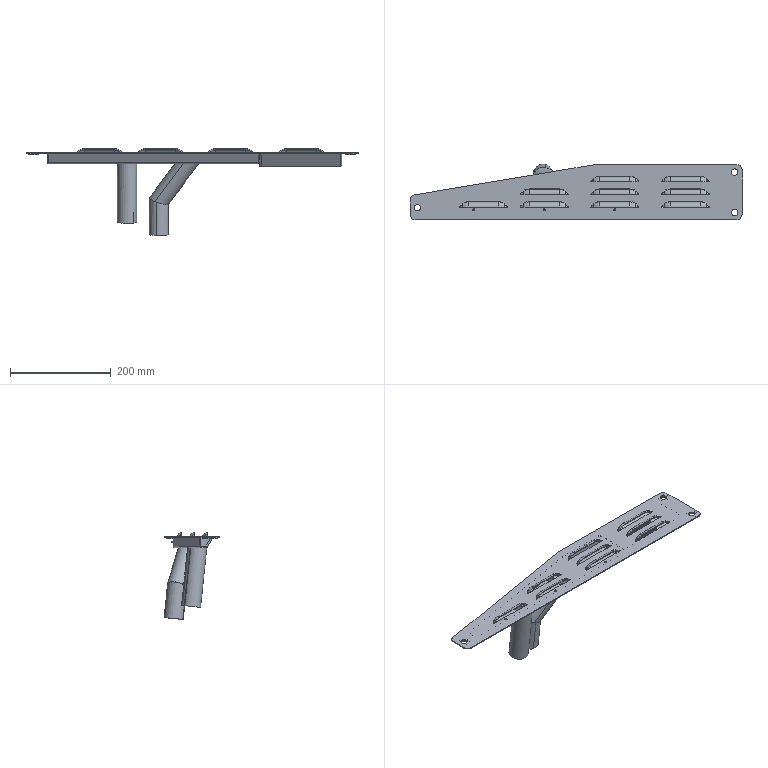Part | SolidWorks | features BaseBody 11, ICE 1 | 11 solids | 588 faces | box 659 x 110.627 x 172.546 mm | volume 240293 mm3 | cylinder 322 | spline 118 | plane 112 | cone 36 | commonest cylinder face diameters 4 x230 20 x13 12.5 x12 2.8 x9 6 x9 16.8 x9